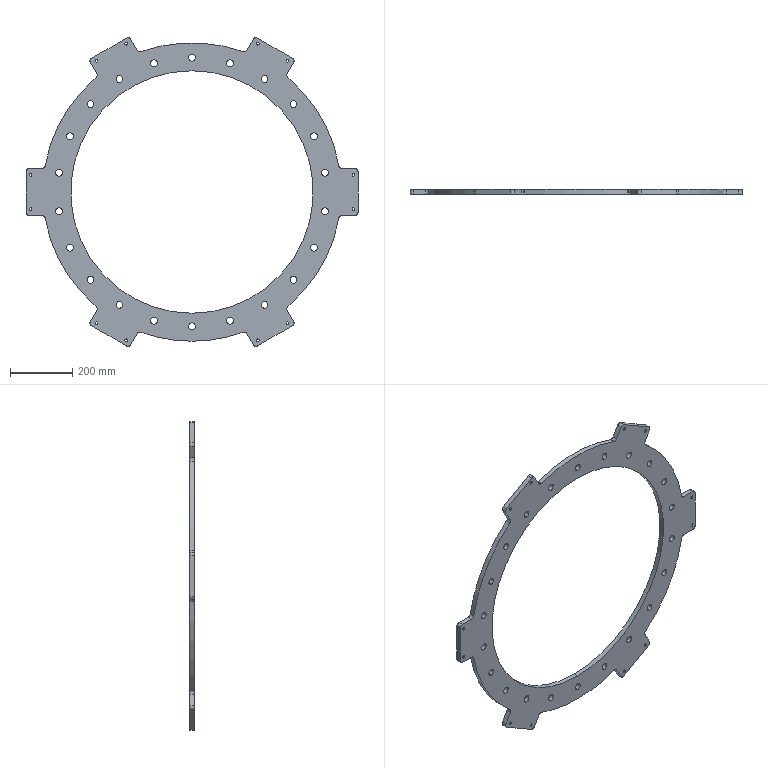Part | SolidWorks | features HoleWzd 2, Extrusion 1, Fillet 1 | 1 solid | 125 faces | box 1068 x 16 x 992.595 mm | volume 4595541 mm3 | cylinder 105 | plane 20 | commonest cylinder face diameters 22 x44 20 x28 8.5 x24 960 x7 780 x2